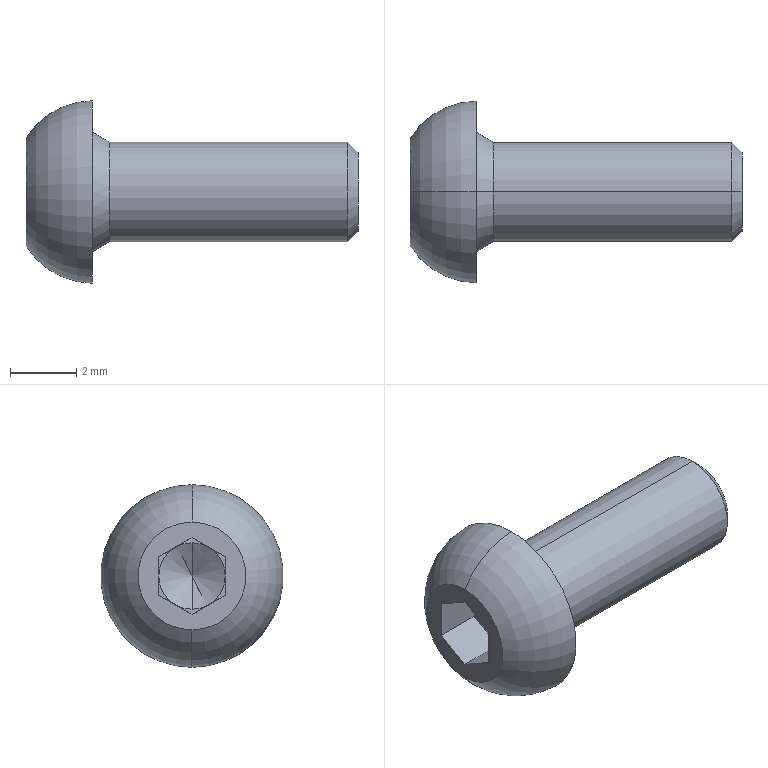Part | NX | features BREP 1 | 1 solid | 25 faces | box 10 x 5.5 x 5.5 mm | volume 88.704 mm3 | plane 15 | cone 6 | cylinder 2 | torus 2 | commonest cylinder face diameters 3 x2
STEP:
#1=CARTESIAN_POINT('',(1.977,0.,0.));
#2=VERTEX_POINT('',#1);
#3=CARTESIAN_POINT('',(1.4,0.,1.));
#4=VERTEX_POINT('',#3);
#5=CARTESIAN_POINT('',(1.4,0.,1.));
#6=DIRECTION('',(-0.5,0.,0.866));
#7=VECTOR('',#6,1000.);
#8=LINE('',#5,#7);
#9=EDGE_CURVE('',#2,#4,#8,.T.);
#10=ORIENTED_EDGE('',*,*,#9,.F.);
#11=CARTESIAN_POINT('',(1.4,0.,-1.));
#12=VERTEX_POINT('',#11);
#13=CARTESIAN_POINT('',(1.4,0.,-1.));
#14=DIRECTION('',(-0.5,0.,-0.866));
#15=VECTOR('',#14,1000.);
#16=LINE('',#13,#15);
#17=EDGE_CURVE('',#2,#12,#16,.T.);
#18=ORIENTED_EDGE('',*,*,#17,.T.);
#19=CARTESIAN_POINT('',(1.4,-0.5,-0.866));
#20=VERTEX_POINT('',#19);
#21=CARTESIAN_POINT('',(1.4,0.,0.));
#22=DIRECTION('',(1.,0.,0.));
#23=DIRECTION('',(0.,0.,1.));
#24=AXIS2_PLACEMENT_3D('',#21,#22,#23);
#25=CIRCLE('',#24,1.);
#26=EDGE_CURVE('',#20,#12,#25,.T.);
#27=ORIENTED_EDGE('',*,*,#26,.F.);
#28=CARTESIAN_POINT('',(1.4,-1.,0.));
#29=VERTEX_POINT('',#28);
#30=CARTESIAN_POINT('',(1.4,0.,0.));
#31=DIRECTION('',(1.,0.,0.));
#32=DIRECTION('',(0.,0.,1.));
#33=AXIS2_PLACEMENT_3D('',#30,#31,#32);
#34=CIRCLE('',#33,1.);
#35=EDGE_CURVE('',#29,#20,#34,.T.);
#36=ORIENTED_EDGE('',*,*,#35,.F.);
#37=CARTESIAN_POINT('',(1.4,-0.5,0.866));
#38=VERTEX_POINT('',#37);
#39=CARTESIAN_POINT('',(1.4,0.,0.));
#40=DIRECTION('',(1.,0.,0.));
#41=DIRECTION('',(0.,0.,1.));
#42=AXIS2_PLACEMENT_3D('',#39,#40,#41);
#43=CIRCLE('',#42,1.);
#44=EDGE_CURVE('',#38,#29,#43,.T.);
#45=ORIENTED_EDGE('',*,*,#44,.F.);
#46=CARTESIAN_POINT('',(1.4,0.,0.));
#47=DIRECTION('',(1.,0.,0.));
#48=DIRECTION('',(0.,0.,1.));
#49=AXIS2_PLACEMENT_3D('',#46,#47,#48);
#50=CIRCLE('',#49,1.);
#51=EDGE_CURVE('',#4,#38,#50,.T.);
#52=ORIENTED_EDGE('',*,*,#51,.F.);
#53=EDGE_LOOP('',(#10,#18,#27,#36,#45,#52));
#54=FACE_BOUND('',#53,.T.);
#55=CARTESIAN_POINT('',(1.4,0.,0.));
#56=DIRECTION('',(-1.,0.,0.));
#57=DIRECTION('',(0.,0.,-1.));
#58=AXIS2_PLACEMENT_3D('',#55,#56,#57);
#59=CONICAL_SURFACE('',#58,1.,1.047);
#60=ADVANCED_FACE('',(#54),#59,.F.);
#61=CARTESIAN_POINT('',(10.,0.,1.194));
#62=VERTEX_POINT('',#61);
#63=CARTESIAN_POINT('',(10.,0.,-1.194));
#64=VERTEX_POINT('',#63);
#65=CARTESIAN_POINT('',(10.,0.,0.));
#66=DIRECTION('',(-1.,0.,0.));
#67=DIRECTION('',(0.,0.,1.));
#68=AXIS2_PLACEMENT_3D('',#65,#66,#67);
#69=CIRCLE('',#68,1.194);
#70=EDGE_CURVE('',#62,#64,#69,.T.);
#71=ORIENTED_EDGE('',*,*,#70,.T.);
#72=CARTESIAN_POINT('',(9.694,0.,-1.5));
#73=VERTEX_POINT('',#72);
#74=CARTESIAN_POINT('',(10.,0.,-1.194));
#75=DIRECTION('',(-0.7071,0.,-0.7071));
#76=VECTOR('',#75,1000.);
#77=LINE('',#74,#76);
#78=EDGE_CURVE('',#64,#73,#77,.T.);
#79=ORIENTED_EDGE('',*,*,#78,.T.);
#80=CARTESIAN_POINT('',(9.694,0.,1.5));
#81=VERTEX_POINT('',#80);
#82=CARTESIAN_POINT('',(9.694,0.,0.));
#83=DIRECTION('',(-1.,0.,0.));
#84=DIRECTION('',(0.,0.,1.));
#85=AXIS2_PLACEMENT_3D('',#82,#83,#84);
#86=CIRCLE('',#85,1.5);
#87=EDGE_CURVE('',#81,#73,#86,.T.);
#88=ORIENTED_EDGE('',*,*,#87,.F.);
#89=CARTESIAN_POINT('',(10.,0.,1.194));
#90=DIRECTION('',(-0.7071,0.,0.7071));
#91=VECTOR('',#90,1000.);
#92=LINE('',#89,#91);
#93=EDGE_CURVE('',#62,#81,#92,.T.);
#94=ORIENTED_EDGE('',*,*,#93,.F.);
#95=EDGE_LOOP('',(#71,#79,#88,#94));
#96=FACE_BOUND('',#95,.T.);
#97=CARTESIAN_POINT('',(10.,0.,0.));
#98=DIRECTION('',(-1.,0.,0.));
#99=DIRECTION('',(0.,0.,-1.));
#100=AXIS2_PLACEMENT_3D('',#97,#98,#99);
#101=CONICAL_SURFACE('',#100,1.194,0.7854);
#102=ADVANCED_FACE('',(#96),#101,.T.);
#103=ORIENTED_EDGE('',*,*,#87,.T.);
#104=CARTESIAN_POINT('',(2.52,0.,-1.5));
#105=VERTEX_POINT('',#104);
#106=CARTESIAN_POINT('',(10.,0.,-1.5));
#107=DIRECTION('',(-1.,0.,0.));
#108=VECTOR('',#107,1000.);
#109=LINE('',#106,#108);
#110=EDGE_CURVE('',#73,#105,#109,.T.);
#111=ORIENTED_EDGE('',*,*,#110,.T.);
#112=CARTESIAN_POINT('',(2.52,0.,1.5));
#113=VERTEX_POINT('',#112);
#114=CARTESIAN_POINT('',(2.52,0.,0.));
#115=DIRECTION('',(-1.,0.,0.));
#116=DIRECTION('',(0.,0.,1.));
#117=AXIS2_PLACEMENT_3D('',#114,#115,#116);
#118=CIRCLE('',#117,1.5);
#119=EDGE_CURVE('',#113,#105,#118,.T.);
#120=ORIENTED_EDGE('',*,*,#119,.F.);
#121=CARTESIAN_POINT('',(10.,0.,1.5));
#122=DIRECTION('',(-1.,0.,0.));
#123=VECTOR('',#122,1000.);
#124=LINE('',#121,#123);
#125=EDGE_CURVE('',#81,#113,#124,.T.);
#126=ORIENTED_EDGE('',*,*,#125,.F.);
#127=EDGE_LOOP('',(#103,#111,#120,#126));
#128=FACE_BOUND('',#127,.T.);
#129=CARTESIAN_POINT('',(10.,0.,0.));
#130=DIRECTION('',(-1.,0.,0.));
#131=DIRECTION('',(0.,0.,-1.));
#132=AXIS2_PLACEMENT_3D('',#129,#130,#131);
#133=CYLINDRICAL_SURFACE('',#132,1.5);
#134=ADVANCED_FACE('',(#128),#133,.T.);
#135=ORIENTED_EDGE('',*,*,#119,.T.);
#136=CARTESIAN_POINT('',(2.,0.,-1.8));
#137=VERTEX_POINT('',#136);
#138=CARTESIAN_POINT('',(2.52,0.,-1.5));
#139=DIRECTION('',(-0.866,0.,-0.5));
#140=VECTOR('',#139,1000.);
#141=LINE('',#138,#140);
#142=EDGE_CURVE('',#105,#137,#141,.T.);
#143=ORIENTED_EDGE('',*,*,#142,.T.);
#144=CARTESIAN_POINT('',(2.,0.,1.8));
#145=VERTEX_POINT('',#144);
#146=CARTESIAN_POINT('',(2.,0.,0.));
#147=DIRECTION('',(-1.,0.,0.));
#148=DIRECTION('',(0.,0.,1.));
#149=AXIS2_PLACEMENT_3D('',#146,#147,#148);
#150=CIRCLE('',#149,1.8);
#151=EDGE_CURVE('',#145,#137,#150,.T.);
#152=ORIENTED_EDGE('',*,*,#151,.F.);
#153=CARTESIAN_POINT('',(2.52,0.,1.5));
#154=DIRECTION('',(-0.866,0.,0.5));
#155=VECTOR('',#154,1000.);
#156=LINE('',#153,#155);
#157=EDGE_CURVE('',#113,#145,#156,.T.);
#158=ORIENTED_EDGE('',*,*,#157,.F.);
#159=EDGE_LOOP('',(#135,#143,#152,#158));
#160=FACE_BOUND('',#159,.T.);
#161=CARTESIAN_POINT('',(2.52,0.,0.));
#162=DIRECTION('',(-1.,0.,0.));
#163=DIRECTION('',(0.,0.,-1.));
#164=AXIS2_PLACEMENT_3D('',#161,#162,#163);
#165=CONICAL_SURFACE('',#164,1.5,0.5236);
#166=ADVANCED_FACE('',(#160),#165,.T.);
#167=CARTESIAN_POINT('',(2.,0.,2.75));
#168=VERTEX_POINT('',#167);
#169=CARTESIAN_POINT('',(2.,0.,-2.75));
#170=VERTEX_POINT('',#169);
#171=CARTESIAN_POINT('',(2.,0.,0.));
#172=DIRECTION('',(-1.,0.,0.));
#173=DIRECTION('',(0.,0.,1.));
#174=AXIS2_PLACEMENT_3D('',#171,#172,#173);
#175=CIRCLE('',#174,2.75);
#176=EDGE_CURVE('',#168,#170,#175,.T.);
#177=ORIENTED_EDGE('',*,*,#176,.T.);
#178=CARTESIAN_POINT('',(0.,0.,-1.625));
#179=VERTEX_POINT('',#178);
#180=CARTESIAN_POINT('',(2.033,0.,-0.3502));
#181=DIRECTION('',(0.,1.,0.));
#182=DIRECTION('',(0.,0.,1.));
#183=AXIS2_PLACEMENT_3D('',#180,#181,#182);
#184=CIRCLE('',#183,2.4);
#185=EDGE_CURVE('',#170,#179,#184,.T.);
#186=ORIENTED_EDGE('',*,*,#185,.T.);
#187=CARTESIAN_POINT('',(0.,0.,1.625));
#188=VERTEX_POINT('',#187);
#189=CARTESIAN_POINT('',(0.,0.,0.));
#190=DIRECTION('',(-1.,0.,0.));
#191=DIRECTION('',(0.,0.,1.));
#192=AXIS2_PLACEMENT_3D('',#189,#190,#191);
#193=CIRCLE('',#192,1.625);
#194=EDGE_CURVE('',#188,#179,#193,.T.);
#195=ORIENTED_EDGE('',*,*,#194,.F.);
#196=CARTESIAN_POINT('',(2.033,0.,0.3502));
#197=DIRECTION('',(0.,-1.,0.));
#198=DIRECTION('',(0.,0.,-1.));
#199=AXIS2_PLACEMENT_3D('',#196,#197,#198);
#200=CIRCLE('',#199,2.4);
#201=EDGE_CURVE('',#168,#188,#200,.T.);
#202=ORIENTED_EDGE('',*,*,#201,.F.);
#203=EDGE_LOOP('',(#177,#186,#195,#202));
#204=FACE_BOUND('',#203,.T.);
#205=CARTESIAN_POINT('',(2.033,0.,0.));
#206=DIRECTION('',(-1.,0.,0.));
#207=DIRECTION('',(0.,0.,-1.));
#208=AXIS2_PLACEMENT_3D('',#205,#206,#207);
#209=DEGENERATE_TOROIDAL_SURFACE('',#208,0.3502,2.4,.T.);
#210=ADVANCED_FACE('',(#204),#209,.T.);
#211=CARTESIAN_POINT('',(0.,-1.,0.5774));
#212=VERTEX_POINT('',#211);
#213=CARTESIAN_POINT('',(0.,0.,1.155));
#214=VERTEX_POINT('',#213);
#215=CARTESIAN_POINT('',(0.,-1.,0.5774));
#216=DIRECTION('',(0.,0.866,0.5));
#217=VECTOR('',#216,1000.);
#218=LINE('',#215,#217);
#219=EDGE_CURVE('',#212,#214,#218,.T.);
#220=ORIENTED_EDGE('',*,*,#219,.F.);
#221=CARTESIAN_POINT('',(0.,-1.,-0.5774));
#222=VERTEX_POINT('',#221);
#223=CARTESIAN_POINT('',(0.,-1.,-0.5774));
#224=DIRECTION('',(0.,0.,1.));
#225=VECTOR('',#224,1000.);
#226=LINE('',#223,#225);
#227=EDGE_CURVE('',#222,#212,#226,.T.);
#228=ORIENTED_EDGE('',*,*,#227,.F.);
#229=CARTESIAN_POINT('',(0.,0.,-1.155));
#230=VERTEX_POINT('',#229);
#231=CARTESIAN_POINT('',(0.,0.,-1.155));
#232=DIRECTION('',(0.,-0.866,0.5));
#233=VECTOR('',#232,1000.);
#234=LINE('',#231,#233);
#235=EDGE_CURVE('',#230,#222,#234,.T.);
#236=ORIENTED_EDGE('',*,*,#235,.F.);
#237=CARTESIAN_POINT('',(0.,1.,-0.5774));
#238=VERTEX_POINT('',#237);
#239=CARTESIAN_POINT('',(0.,1.,-0.5774));
#240=DIRECTION('',(0.,-0.866,-0.5));
#241=VECTOR('',#240,1000.);
#242=LINE('',#239,#241);
#243=EDGE_CURVE('',#238,#230,#242,.T.);
#244=ORIENTED_EDGE('',*,*,#243,.F.);
#245=CARTESIAN_POINT('',(0.,1.,0.5774));
#246=VERTEX_POINT('',#245);
#247=CARTESIAN_POINT('',(0.,1.,0.5774));
#248=DIRECTION('',(0.,0.,-1.));
#249=VECTOR('',#248,1000.);
#250=LINE('',#247,#249);
#251=EDGE_CURVE('',#246,#238,#250,.T.);
#252=ORIENTED_EDGE('',*,*,#251,.F.);
#253=CARTESIAN_POINT('',(0.,0.,1.155));
#254=DIRECTION('',(0.,0.866,-0.5));
#255=VECTOR('',#254,1000.);
#256=LINE('',#253,#255);
#257=EDGE_CURVE('',#214,#246,#256,.T.);
#258=ORIENTED_EDGE('',*,*,#257,.F.);
#259=EDGE_LOOP('',(#220,#228,#236,#244,#252,#258));
#260=FACE_BOUND('',#259,.T.);
#261=ORIENTED_EDGE('',*,*,#194,.T.);
#262=CARTESIAN_POINT('',(0.,0.,0.));
#263=DIRECTION('',(-1.,0.,0.));
#264=DIRECTION('',(0.,0.,1.));
#265=AXIS2_PLACEMENT_3D('',#262,#263,#264);
#266=CIRCLE('',#265,1.625);
#267=EDGE_CURVE('',#179,#188,#266,.T.);
#268=ORIENTED_EDGE('',*,*,#267,.T.);
#269=EDGE_LOOP('',(#261,#268));
#270=FACE_BOUND('',#269,.T.);
#271=CARTESIAN_POINT('',(0.,0.5,0.));
#272=DIRECTION('',(1.,0.,0.));
#273=DIRECTION('',(0.,0.,1.));
#274=AXIS2_PLACEMENT_3D('',#271,#272,#273);
#275=PLANE('',#274);
#276=ADVANCED_FACE('',(#260,#270),#275,.F.);
#277=ORIENTED_EDGE('',*,*,#185,.F.);
#278=CARTESIAN_POINT('',(2.,0.,0.));
#279=DIRECTION('',(-1.,0.,0.));
#280=DIRECTION('',(0.,0.,1.));
#281=AXIS2_PLACEMENT_3D('',#278,#279,#280);
#282=CIRCLE('',#281,2.75);
#283=EDGE_CURVE('',#170,#168,#282,.T.);
#284=ORIENTED_EDGE('',*,*,#283,.T.);
#285=ORIENTED_EDGE('',*,*,#201,.T.);
#286=ORIENTED_EDGE('',*,*,#267,.F.);
#287=EDGE_LOOP('',(#277,#284,#285,#286));
#288=FACE_BOUND('',#287,.T.);
#289=CARTESIAN_POINT('',(2.033,0.,0.));
#290=DIRECTION('',(-1.,0.,0.));
#291=DIRECTION('',(0.,0.,-1.));
#292=AXIS2_PLACEMENT_3D('',#289,#290,#291);
#293=DEGENERATE_TOROIDAL_SURFACE('',#292,0.3502,2.4,.T.);
#294=ADVANCED_FACE('',(#288),#293,.T.);
#295=ORIENTED_EDGE('',*,*,#176,.F.);
#296=ORIENTED_EDGE('',*,*,#283,.F.);
#297=EDGE_LOOP('',(#295,#296));
#298=FACE_BOUND('',#297,.T.);
#299=ORIENTED_EDGE('',*,*,#151,.T.);
#300=CARTESIAN_POINT('',(2.,0.,0.));
#301=DIRECTION('',(-1.,0.,0.));
#302=DIRECTION('',(0.,0.,1.));
#303=AXIS2_PLACEMENT_3D('',#300,#301,#302);
#304=CIRCLE('',#303,1.8);
#305=EDGE_CURVE('',#137,#145,#304,.T.);
#306=ORIENTED_EDGE('',*,*,#305,.T.);
#307=EDGE_LOOP('',(#299,#306));
#308=FACE_BOUND('',#307,.T.);
#309=CARTESIAN_POINT('',(2.,2.75,0.));
#310=DIRECTION('',(-1.,0.,0.));
#311=DIRECTION('',(0.,0.,-1.));
#312=AXIS2_PLACEMENT_3D('',#309,#310,#311);
#313=PLANE('',#312);
#314=ADVANCED_FACE('',(#298,#308),#313,.F.);
#315=ORIENTED_EDGE('',*,*,#142,.F.);
#316=CARTESIAN_POINT('',(2.52,0.,0.));
#317=DIRECTION('',(-1.,0.,0.));
#318=DIRECTION('',(0.,0.,1.));
#319=AXIS2_PLACEMENT_3D('',#316,#317,#318);
#320=CIRCLE('',#319,1.5);
#321=EDGE_CURVE('',#105,#113,#320,.T.);
#322=ORIENTED_EDGE('',*,*,#321,.T.);
#323=ORIENTED_EDGE('',*,*,#157,.T.);
#324=ORIENTED_EDGE('',*,*,#305,.F.);
#325=EDGE_LOOP('',(#315,#322,#323,#324));
#326=FACE_BOUND('',#325,.T.);
#327=CARTESIAN_POINT('',(2.52,0.,0.));
#328=DIRECTION('',(-1.,0.,0.));
#329=DIRECTION('',(0.,0.,-1.));
#330=AXIS2_PLACEMENT_3D('',#327,#328,#329);
#331=CONICAL_SURFACE('',#330,1.5,0.5236);
#332=ADVANCED_FACE('',(#326),#331,.T.);
#333=ORIENTED_EDGE('',*,*,#110,.F.);
#334=CARTESIAN_POINT('',(9.694,0.,0.));
#335=DIRECTION('',(-1.,0.,0.));
#336=DIRECTION('',(0.,0.,1.));
#337=AXIS2_PLACEMENT_3D('',#334,#335,#336);
#338=CIRCLE('',#337,1.5);
#339=EDGE_CURVE('',#73,#81,#338,.T.);
#340=ORIENTED_EDGE('',*,*,#339,.T.);
#341=ORIENTED_EDGE('',*,*,#125,.T.);
#342=ORIENTED_EDGE('',*,*,#321,.F.);
#343=EDGE_LOOP('',(#333,#340,#341,#342));
#344=FACE_BOUND('',#343,.T.);
#345=CARTESIAN_POINT('',(10.,0.,0.));
#346=DIRECTION('',(-1.,0.,0.));
#347=DIRECTION('',(0.,0.,-1.));
#348=AXIS2_PLACEMENT_3D('',#345,#346,#347);
#349=CYLINDRICAL_SURFACE('',#348,1.5);
#350=ADVANCED_FACE('',(#344),#349,.T.);
#351=ORIENTED_EDGE('',*,*,#78,.F.);
#352=CARTESIAN_POINT('',(10.,0.,0.));
#353=DIRECTION('',(-1.,0.,0.));
#354=DIRECTION('',(0.,0.,1.));
#355=AXIS2_PLACEMENT_3D('',#352,#353,#354);
#356=CIRCLE('',#355,1.194);
#357=EDGE_CURVE('',#64,#62,#356,.T.);
#358=ORIENTED_EDGE('',*,*,#357,.T.);
#359=ORIENTED_EDGE('',*,*,#93,.T.);
#360=ORIENTED_EDGE('',*,*,#339,.F.);
#361=EDGE_LOOP('',(#351,#358,#359,#360));
#362=FACE_BOUND('',#361,.T.);
#363=CARTESIAN_POINT('',(10.,0.,0.));
#364=DIRECTION('',(-1.,0.,0.));
#365=DIRECTION('',(0.,0.,-1.));
#366=AXIS2_PLACEMENT_3D('',#363,#364,#365);
#367=CONICAL_SURFACE('',#366,1.194,0.7854);
#368=ADVANCED_FACE('',(#362),#367,.T.);
#369=ORIENTED_EDGE('',*,*,#70,.F.);
#370=ORIENTED_EDGE('',*,*,#357,.F.);
#371=EDGE_LOOP('',(#369,#370));
#372=FACE_BOUND('',#371,.T.);
#373=CARTESIAN_POINT('',(10.,1.194,0.));
#374=DIRECTION('',(-1.,0.,0.));
#375=DIRECTION('',(0.,0.,-1.));
#376=AXIS2_PLACEMENT_3D('',#373,#374,#375);
#377=PLANE('',#376);
#378=ADVANCED_FACE('',(#372),#377,.F.);
#379=ORIENTED_EDGE('',*,*,#44,.T.);
#380=CARTESIAN_POINT('',(1.4,-1.,0.5774));
#381=VERTEX_POINT('',#380);
#382=CARTESIAN_POINT('',(1.4,-1.,-0.5774));
#383=DIRECTION('',(0.,0.,1.));
#384=VECTOR('',#383,1000.);
#385=LINE('',#382,#384);
#386=EDGE_CURVE('',#29,#381,#385,.T.);
#387=ORIENTED_EDGE('',*,*,#386,.T.);
#388=CARTESIAN_POINT('',(1.4,-1.,0.5774));
#389=DIRECTION('',(0.,0.866,0.5));
#390=VECTOR('',#389,1000.);
#391=LINE('',#388,#390);
#392=EDGE_CURVE('',#381,#38,#391,.T.);
#393=ORIENTED_EDGE('',*,*,#392,.T.);
#394=EDGE_LOOP('',(#379,#387,#393));
#395=FACE_BOUND('',#394,.T.);
#396=CARTESIAN_POINT('',(1.4,0.,0.));
#397=DIRECTION('',(-1.,0.,0.));
#398=DIRECTION('',(0.,0.,-1.));
#399=AXIS2_PLACEMENT_3D('',#396,#397,#398);
#400=PLANE('',#399);
#401=ADVANCED_FACE('',(#395),#400,.T.);
#402=ORIENTED_EDGE('',*,*,#35,.T.);
#403=CARTESIAN_POINT('',(1.4,-1.,-0.5774));
#404=VERTEX_POINT('',#403);
#405=CARTESIAN_POINT('',(1.4,0.,-1.155));
#406=DIRECTION('',(0.,-0.866,0.5));
#407=VECTOR('',#406,1000.);
#408=LINE('',#405,#407);
#409=EDGE_CURVE('',#20,#404,#408,.T.);
#410=ORIENTED_EDGE('',*,*,#409,.T.);
#411=CARTESIAN_POINT('',(1.4,-1.,-0.5774));
#412=DIRECTION('',(0.,0.,1.));
#413=VECTOR('',#412,1000.);
#414=LINE('',#411,#413);
#415=EDGE_CURVE('',#404,#29,#414,.T.);
#416=ORIENTED_EDGE('',*,*,#415,.T.);
#417=EDGE_LOOP('',(#402,#410,#416));
#418=FACE_BOUND('',#417,.T.);
#419=CARTESIAN_POINT('',(1.4,0.,0.));
#420=DIRECTION('',(-1.,0.,0.));
#421=DIRECTION('',(0.,0.,-1.));
#422=AXIS2_PLACEMENT_3D('',#419,#420,#421);
#423=PLANE('',#422);
#424=ADVANCED_FACE('',(#418),#423,.T.);
#425=ORIENTED_EDGE('',*,*,#26,.T.);
#426=CARTESIAN_POINT('',(1.4,0.5,-0.866));
#427=VERTEX_POINT('',#426);
#428=CARTESIAN_POINT('',(1.4,0.,0.));
#429=DIRECTION('',(1.,0.,0.));
#430=DIRECTION('',(0.,0.,1.));
#431=AXIS2_PLACEMENT_3D('',#428,#429,#430);
#432=CIRCLE('',#431,1.);
#433=EDGE_CURVE('',#12,#427,#432,.T.);
#434=ORIENTED_EDGE('',*,*,#433,.T.);
#435=CARTESIAN_POINT('',(1.4,0.,-1.155));
#436=VERTEX_POINT('',#435);
#437=CARTESIAN_POINT('',(1.4,1.,-0.5774));
#438=DIRECTION('',(0.,-0.866,-0.5));
#439=VECTOR('',#438,1000.);
#440=LINE('',#437,#439);
#441=EDGE_CURVE('',#427,#436,#440,.T.);
#442=ORIENTED_EDGE('',*,*,#441,.T.);
#443=CARTESIAN_POINT('',(1.4,0.,-1.155));
#444=DIRECTION('',(0.,-0.866,0.5));
#445=VECTOR('',#444,1000.);
#446=LINE('',#443,#445);
#447=EDGE_CURVE('',#436,#20,#446,.T.);
#448=ORIENTED_EDGE('',*,*,#447,.T.);
#449=EDGE_LOOP('',(#425,#434,#442,#448));
#450=FACE_BOUND('',#449,.T.);
#451=CARTESIAN_POINT('',(1.4,0.,0.));
#452=DIRECTION('',(-1.,0.,0.));
#453=DIRECTION('',(0.,0.,-1.));
#454=AXIS2_PLACEMENT_3D('',#451,#452,#453);
#455=PLANE('',#454);
#456=ADVANCED_FACE('',(#450),#455,.T.);
#457=CARTESIAN_POINT('',(1.4,1.,0.));
#458=VERTEX_POINT('',#457);
#459=CARTESIAN_POINT('',(1.4,0.,0.));
#460=DIRECTION('',(1.,0.,0.));
#461=DIRECTION('',(0.,0.,1.));
#462=AXIS2_PLACEMENT_3D('',#459,#460,#461);
#463=CIRCLE('',#462,1.);
#464=EDGE_CURVE('',#427,#458,#463,.T.);
#465=ORIENTED_EDGE('',*,*,#464,.T.);
#466=CARTESIAN_POINT('',(1.4,1.,-0.5774));
#467=VERTEX_POINT('',#466);
#468=CARTESIAN_POINT('',(1.4,1.,0.5774));
#469=DIRECTION('',(0.,0.,-1.));
#470=VECTOR('',#469,1000.);
#471=LINE('',#468,#470);
#472=EDGE_CURVE('',#458,#467,#471,.T.);
#473=ORIENTED_EDGE('',*,*,#472,.T.);
#474=CARTESIAN_POINT('',(1.4,1.,-0.5774));
#475=DIRECTION('',(0.,-0.866,-0.5));
#476=VECTOR('',#475,1000.);
#477=LINE('',#474,#476);
#478=EDGE_CURVE('',#467,#427,#477,.T.);
#479=ORIENTED_EDGE('',*,*,#478,.T.);
#480=EDGE_LOOP('',(#465,#473,#479));
#481=FACE_BOUND('',#480,.T.);
#482=CARTESIAN_POINT('',(1.4,0.,0.));
#483=DIRECTION('',(-1.,0.,0.));
#484=DIRECTION('',(0.,0.,-1.));
#485=AXIS2_PLACEMENT_3D('',#482,#483,#484);
#486=PLANE('',#485);
#487=ADVANCED_FACE('',(#481),#486,.T.);
#488=CARTESIAN_POINT('',(1.4,0.5,0.866));
#489=VERTEX_POINT('',#488);
#490=CARTESIAN_POINT('',(1.4,0.,0.));
#491=DIRECTION('',(-1.,0.,0.));
#492=DIRECTION('',(0.,0.,1.));
#493=AXIS2_PLACEMENT_3D('',#490,#491,#492);
#494=CIRCLE('',#493,1.);
#495=EDGE_CURVE('',#489,#458,#494,.T.);
#496=ORIENTED_EDGE('',*,*,#495,.F.);
#497=CARTESIAN_POINT('',(1.4,1.,0.5774));
#498=VERTEX_POINT('',#497);
#499=CARTESIAN_POINT('',(1.4,0.,1.155));
#500=DIRECTION('',(0.,0.866,-0.5));
#501=VECTOR('',#500,1000.);
#502=LINE('',#499,#501);
#503=EDGE_CURVE('',#489,#498,#502,.T.);
#504=ORIENTED_EDGE('',*,*,#503,.T.);
#505=CARTESIAN_POINT('',(1.4,1.,0.5774));
#506=DIRECTION('',(0.,0.,-1.));
#507=VECTOR('',#506,1000.);
#508=LINE('',#505,#507);
#509=EDGE_CURVE('',#498,#458,#508,.T.);
#510=ORIENTED_EDGE('',*,*,#509,.T.);
#511=EDGE_LOOP('',(#496,#504,#510));
#512=FACE_BOUND('',#511,.T.);
#513=CARTESIAN_POINT('',(1.4,0.,0.));
#514=DIRECTION('',(-1.,0.,0.));
#515=DIRECTION('',(0.,0.,-1.));
#516=AXIS2_PLACEMENT_3D('',#513,#514,#515);
#517=PLANE('',#516);
#518=ADVANCED_FACE('',(#512),#517,.T.);
#519=CARTESIAN_POINT('',(1.4,0.,0.));
#520=DIRECTION('',(1.,0.,0.));
#521=DIRECTION('',(0.,0.,1.));
#522=AXIS2_PLACEMENT_3D('',#519,#520,#521);
#523=CIRCLE('',#522,1.);
#524=EDGE_CURVE('',#489,#4,#523,.T.);
#525=ORIENTED_EDGE('',*,*,#524,.T.);
#526=ORIENTED_EDGE('',*,*,#51,.T.);
#527=CARTESIAN_POINT('',(1.4,0.,1.155));
#528=VERTEX_POINT('',#527);
#529=CARTESIAN_POINT('',(1.4,-1.,0.5774));
#530=DIRECTION('',(0.,0.866,0.5));
#531=VECTOR('',#530,1000.);
#532=LINE('',#529,#531);
#533=EDGE_CURVE('',#38,#528,#532,.T.);
#534=ORIENTED_EDGE('',*,*,#533,.T.);
#535=CARTESIAN_POINT('',(1.4,0.,1.155));
#536=DIRECTION('',(0.,0.866,-0.5));
#537=VECTOR('',#536,1000.);
#538=LINE('',#535,#537);
#539=EDGE_CURVE('',#528,#489,#538,.T.);
#540=ORIENTED_EDGE('',*,*,#539,.T.);
#541=EDGE_LOOP('',(#525,#526,#534,#540));
#542=FACE_BOUND('',#541,.T.);
#543=CARTESIAN_POINT('',(1.4,0.,0.));
#544=DIRECTION('',(-1.,0.,0.));
#545=DIRECTION('',(0.,0.,-1.));
#546=AXIS2_PLACEMENT_3D('',#543,#544,#545);
#547=PLANE('',#546);
#548=ADVANCED_FACE('',(#542),#547,.T.);
#549=ORIENTED_EDGE('',*,*,#227,.T.);
#550=CARTESIAN_POINT('',(1.4,-1.,0.5774));
#551=DIRECTION('',(-1.,0.,0.));
#552=VECTOR('',#551,1000.);
#553=LINE('',#550,#552);
#554=EDGE_CURVE('',#381,#212,#553,.T.);
#555=ORIENTED_EDGE('',*,*,#554,.F.);
#556=ORIENTED_EDGE('',*,*,#386,.F.);
#557=ORIENTED_EDGE('',*,*,#415,.F.);
#558=CARTESIAN_POINT('',(1.4,-1.,-0.5774));
#559=DIRECTION('',(-1.,0.,0.));
#560=VECTOR('',#559,1000.);
#561=LINE('',#558,#560);
#562=EDGE_CURVE('',#404,#222,#561,.T.);
#563=ORIENTED_EDGE('',*,*,#562,.T.);
#564=EDGE_LOOP('',(#549,#555,#556,#557,#563));
#565=FACE_BOUND('',#564,.T.);
#566=CARTESIAN_POINT('',(1.4,-1.,-0.5774));
#567=DIRECTION('',(0.,-1.,0.));
#568=DIRECTION('',(0.,0.,1.));
#569=AXIS2_PLACEMENT_3D('',#566,#567,#568);
#570=PLANE('',#569);
#571=ADVANCED_FACE('',(#565),#570,.F.);
#572=ORIENTED_EDGE('',*,*,#235,.T.);
#573=ORIENTED_EDGE('',*,*,#562,.F.);
#574=ORIENTED_EDGE('',*,*,#409,.F.);
#575=ORIENTED_EDGE('',*,*,#447,.F.);
#576=CARTESIAN_POINT('',(1.4,0.,-1.155));
#577=DIRECTION('',(-1.,0.,0.));
#578=VECTOR('',#577,1000.);
#579=LINE('',#576,#578);
#580=EDGE_CURVE('',#436,#230,#579,.T.);
#581=ORIENTED_EDGE('',*,*,#580,.T.);
#582=EDGE_LOOP('',(#572,#573,#574,#575,#581));
#583=FACE_BOUND('',#582,.T.);
#584=CARTESIAN_POINT('',(1.4,0.,-1.155));
#585=DIRECTION('',(0.,-0.5,-0.866));
#586=DIRECTION('',(0.,-0.866,0.5));
#587=AXIS2_PLACEMENT_3D('',#584,#585,#586);
#588=PLANE('',#587);
#589=ADVANCED_FACE('',(#583),#588,.F.);
#590=ORIENTED_EDGE('',*,*,#243,.T.);
#591=ORIENTED_EDGE('',*,*,#580,.F.);
#592=ORIENTED_EDGE('',*,*,#441,.F.);
#593=ORIENTED_EDGE('',*,*,#478,.F.);
#594=CARTESIAN_POINT('',(1.4,1.,-0.5774));
#595=DIRECTION('',(-1.,0.,0.));
#596=VECTOR('',#595,1000.);
#597=LINE('',#594,#596);
#598=EDGE_CURVE('',#467,#238,#597,.T.);
#599=ORIENTED_EDGE('',*,*,#598,.T.);
#600=EDGE_LOOP('',(#590,#591,#592,#593,#599));
#601=FACE_BOUND('',#600,.T.);
#602=CARTESIAN_POINT('',(1.4,1.,-0.5774));
#603=DIRECTION('',(0.,0.5,-0.866));
#604=DIRECTION('',(0.,-0.866,-0.5));
#605=AXIS2_PLACEMENT_3D('',#602,#603,#604);
#606=PLANE('',#605);
#607=ADVANCED_FACE('',(#601),#606,.F.);
#608=ORIENTED_EDGE('',*,*,#251,.T.);
#609=ORIENTED_EDGE('',*,*,#598,.F.);
#610=ORIENTED_EDGE('',*,*,#472,.F.);
#611=ORIENTED_EDGE('',*,*,#509,.F.);
#612=CARTESIAN_POINT('',(1.4,1.,0.5774));
#613=DIRECTION('',(-1.,0.,0.));
#614=VECTOR('',#613,1000.);
#615=LINE('',#612,#614);
#616=EDGE_CURVE('',#498,#246,#615,.T.);
#617=ORIENTED_EDGE('',*,*,#616,.T.);
#618=EDGE_LOOP('',(#608,#609,#610,#611,#617));
#619=FACE_BOUND('',#618,.T.);
#620=CARTESIAN_POINT('',(1.4,1.,0.5774));
#621=DIRECTION('',(0.,1.,0.));
#622=DIRECTION('',(0.,0.,-1.));
#623=AXIS2_PLACEMENT_3D('',#620,#621,#622);
#624=PLANE('',#623);
#625=ADVANCED_FACE('',(#619),#624,.F.);
#626=ORIENTED_EDGE('',*,*,#257,.T.);
#627=ORIENTED_EDGE('',*,*,#616,.F.);
#628=ORIENTED_EDGE('',*,*,#503,.F.);
#629=ORIENTED_EDGE('',*,*,#539,.F.);
#630=CARTESIAN_POINT('',(1.4,0.,1.155));
#631=DIRECTION('',(-1.,0.,0.));
#632=VECTOR('',#631,1000.);
#633=LINE('',#630,#632);
#634=EDGE_CURVE('',#528,#214,#633,.T.);
#635=ORIENTED_EDGE('',*,*,#634,.T.);
#636=EDGE_LOOP('',(#626,#627,#628,#629,#635));
#637=FACE_BOUND('',#636,.T.);
#638=CARTESIAN_POINT('',(1.4,0.,1.155));
#639=DIRECTION('',(0.,0.5,0.866));
#640=DIRECTION('',(0.,0.866,-0.5));
#641=AXIS2_PLACEMENT_3D('',#638,#639,#640);
#642=PLANE('',#641);
#643=ADVANCED_FACE('',(#637),#642,.F.);
#644=ORIENTED_EDGE('',*,*,#219,.T.);
#645=ORIENTED_EDGE('',*,*,#634,.F.);
#646=ORIENTED_EDGE('',*,*,#533,.F.);
#647=ORIENTED_EDGE('',*,*,#392,.F.);
#648=ORIENTED_EDGE('',*,*,#554,.T.);
#649=EDGE_LOOP('',(#644,#645,#646,#647,#648));
#650=FACE_BOUND('',#649,.T.);
#651=CARTESIAN_POINT('',(1.4,-1.,0.5774));
#652=DIRECTION('',(0.,-0.5,0.866));
#653=DIRECTION('',(0.,0.866,0.5));
#654=AXIS2_PLACEMENT_3D('',#651,#652,#653);
#655=PLANE('',#654);
#656=ADVANCED_FACE('',(#650),#655,.F.);
#657=ORIENTED_EDGE('',*,*,#17,.F.);
#658=ORIENTED_EDGE('',*,*,#9,.T.);
#659=ORIENTED_EDGE('',*,*,#524,.F.);
#660=ORIENTED_EDGE('',*,*,#495,.T.);
#661=ORIENTED_EDGE('',*,*,#464,.F.);
#662=ORIENTED_EDGE('',*,*,#433,.F.);
#663=EDGE_LOOP('',(#657,#658,#659,#660,#661,#662));
#664=FACE_BOUND('',#663,.T.);
#665=CARTESIAN_POINT('',(1.4,0.,0.));
#666=DIRECTION('',(-1.,0.,0.));
#667=DIRECTION('',(0.,0.,-1.));
#668=AXIS2_PLACEMENT_3D('',#665,#666,#667);
#669=CONICAL_SURFACE('',#668,1.,1.047);
#670=ADVANCED_FACE('',(#664),#669,.F.);
#671=CLOSED_SHELL('',(#60,#102,#134,#166,#210,#276,#294,#314,#332,#350,#368,#378,#401,#424,#456,#487,#518,#548,#571,#589,#607,#625,#643,#656,#670));
#672=MANIFOLD_SOLID_BREP('',#671);
#673=(LENGTH_UNIT()NAMED_UNIT(*)SI_UNIT(.MILLI.,.METRE.));
#674=UNCERTAINTY_MEASURE_WITH_UNIT(LENGTH_MEASURE(0.00001),#673,'','');
#675=(NAMED_UNIT(*)PLANE_ANGLE_UNIT()SI_UNIT($,.RADIAN.));
#676=(NAMED_UNIT(*)SI_UNIT($,.STERADIAN.)SOLID_ANGLE_UNIT());
#677=(GEOMETRIC_REPRESENTATION_CONTEXT(3)GLOBAL_UNCERTAINTY_ASSIGNED_CONTEXT((#674))GLOBAL_UNIT_ASSIGNED_CONTEXT((#673,#675,#676))REPRESENTATION_CONTEXT('',''));
#678=ADVANCED_BREP_SHAPE_REPRESENTATION('',(#672),#677);